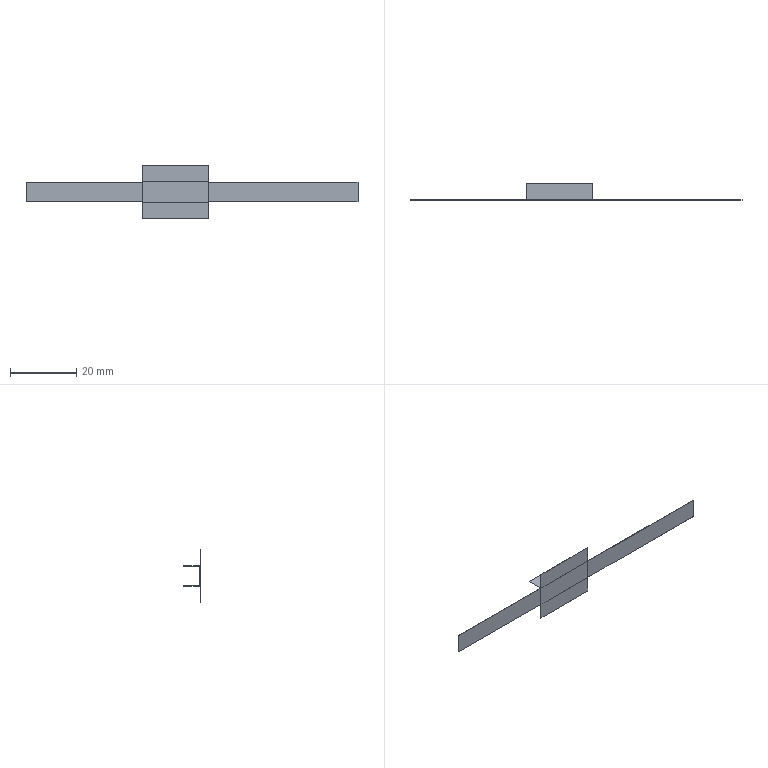Part | SolidWorks | features ICE 2, ExtruThin 1 | 1 solid | 22 faces | box 100 x 5.02 x 16 mm | volume 70.4 mm3 | plane 22
STEP:
#1=CARTESIAN_POINT('',(35.,0.05,3.));
#2=VERTEX_POINT('',#1);
#3=CARTESIAN_POINT('',(35.,-0.05,3.));
#4=VERTEX_POINT('',#3);
#5=CARTESIAN_POINT('',(35.,4.95,3.));
#6=DIRECTION('',(0.,-1.,0.));
#7=VECTOR('',#6,1000.);
#8=LINE('',#5,#7);
#9=EDGE_CURVE('',#2,#4,#8,.T.);
#10=ORIENTED_EDGE('',*,*,#9,.F.);
#11=CARTESIAN_POINT('',(0.,0.05,3.));
#12=VERTEX_POINT('',#11);
#13=CARTESIAN_POINT('',(0.,0.05,3.));
#14=DIRECTION('',(1.,0.,0.));
#15=VECTOR('',#14,1000.);
#16=LINE('',#13,#15);
#17=EDGE_CURVE('',#12,#2,#16,.T.);
#18=ORIENTED_EDGE('',*,*,#17,.F.);
#19=CARTESIAN_POINT('',(0.,-0.05,3.));
#20=VERTEX_POINT('',#19);
#21=CARTESIAN_POINT('',(0.,-0.05,3.));
#22=DIRECTION('',(0.,1.,0.));
#23=VECTOR('',#22,1000.);
#24=LINE('',#21,#23);
#25=EDGE_CURVE('',#20,#12,#24,.T.);
#26=ORIENTED_EDGE('',*,*,#25,.F.);
#27=CARTESIAN_POINT('',(0.,-0.05,3.));
#28=DIRECTION('',(1.,0.,0.));
#29=VECTOR('',#28,1000.);
#30=LINE('',#27,#29);
#31=EDGE_CURVE('',#20,#4,#30,.T.);
#32=ORIENTED_EDGE('',*,*,#31,.T.);
#33=EDGE_LOOP('',(#10,#18,#26,#32));
#34=FACE_OUTER_BOUND('',#33,.T.);
#35=CARTESIAN_POINT('',(100.,-0.05,3.));
#36=DIRECTION('',(0.,0.,-1.));
#37=DIRECTION('',(-1.,0.,0.));
#38=AXIS2_PLACEMENT_3D('',#35,#36,#37);
#39=PLANE('',#38);
#40=ADVANCED_FACE('',(#34),#39,.F.);
#41=CARTESIAN_POINT('',(55.,0.05,3.));
#42=VERTEX_POINT('',#41);
#43=CARTESIAN_POINT('',(55.,-0.05,3.));
#44=VERTEX_POINT('',#43);
#45=CARTESIAN_POINT('',(55.,4.95,3.));
#46=DIRECTION('',(0.,-1.,0.));
#47=VECTOR('',#46,1000.);
#48=LINE('',#45,#47);
#49=EDGE_CURVE('',#42,#44,#48,.T.);
#50=ORIENTED_EDGE('',*,*,#49,.T.);
#51=CARTESIAN_POINT('',(100.,-0.05,3.));
#52=VERTEX_POINT('',#51);
#53=CARTESIAN_POINT('',(0.,-0.05,3.));
#54=DIRECTION('',(1.,0.,0.));
#55=VECTOR('',#54,1000.);
#56=LINE('',#53,#55);
#57=EDGE_CURVE('',#44,#52,#56,.T.);
#58=ORIENTED_EDGE('',*,*,#57,.T.);
#59=CARTESIAN_POINT('',(100.,0.05,3.));
#60=VERTEX_POINT('',#59);
#61=CARTESIAN_POINT('',(100.,0.05,3.));
#62=DIRECTION('',(0.,-1.,0.));
#63=VECTOR('',#62,1000.);
#64=LINE('',#61,#63);
#65=EDGE_CURVE('',#60,#52,#64,.T.);
#66=ORIENTED_EDGE('',*,*,#65,.F.);
#67=CARTESIAN_POINT('',(0.,0.05,3.));
#68=DIRECTION('',(1.,0.,0.));
#69=VECTOR('',#68,1000.);
#70=LINE('',#67,#69);
#71=EDGE_CURVE('',#42,#60,#70,.T.);
#72=ORIENTED_EDGE('',*,*,#71,.F.);
#73=EDGE_LOOP('',(#50,#58,#66,#72));
#74=FACE_OUTER_BOUND('',#73,.T.);
#75=CARTESIAN_POINT('',(100.,-0.05,3.));
#76=DIRECTION('',(0.,0.,-1.));
#77=DIRECTION('',(-1.,0.,0.));
#78=AXIS2_PLACEMENT_3D('',#75,#76,#77);
#79=PLANE('',#78);
#80=ADVANCED_FACE('',(#74),#79,.F.);
#81=CARTESIAN_POINT('',(55.,-0.05,3.02));
#82=VERTEX_POINT('',#81);
#83=CARTESIAN_POINT('',(55.,-0.05,8.));
#84=VERTEX_POINT('',#83);
#85=CARTESIAN_POINT('',(55.,-0.05,-8.));
#86=DIRECTION('',(0.,0.,1.));
#87=VECTOR('',#86,1000.);
#88=LINE('',#85,#87);
#89=EDGE_CURVE('',#82,#84,#88,.T.);
#90=ORIENTED_EDGE('',*,*,#89,.F.);
#91=CARTESIAN_POINT('',(35.,-0.05,3.02));
#92=VERTEX_POINT('',#91);
#93=CARTESIAN_POINT('',(35.,-0.05,3.02));
#94=DIRECTION('',(1.,0.,0.));
#95=VECTOR('',#94,1000.);
#96=LINE('',#93,#95);
#97=EDGE_CURVE('',#92,#82,#96,.T.);
#98=ORIENTED_EDGE('',*,*,#97,.F.);
#99=CARTESIAN_POINT('',(35.,-0.05,8.));
#100=VERTEX_POINT('',#99);
#101=CARTESIAN_POINT('',(35.,-0.05,-8.));
#102=DIRECTION('',(0.,0.,-1.));
#103=VECTOR('',#102,1000.);
#104=LINE('',#101,#103);
#105=EDGE_CURVE('',#100,#92,#104,.T.);
#106=ORIENTED_EDGE('',*,*,#105,.F.);
#107=CARTESIAN_POINT('',(35.,-0.05,8.));
#108=DIRECTION('',(-1.,0.,0.));
#109=VECTOR('',#108,1000.);
#110=LINE('',#107,#109);
#111=EDGE_CURVE('',#84,#100,#110,.T.);
#112=ORIENTED_EDGE('',*,*,#111,.F.);
#113=EDGE_LOOP('',(#90,#98,#106,#112));
#114=FACE_OUTER_BOUND('',#113,.T.);
#115=CARTESIAN_POINT('',(55.,-0.05,8.));
#116=DIRECTION('',(0.,1.,0.));
#117=DIRECTION('',(0.,0.,1.));
#118=AXIS2_PLACEMENT_3D('',#115,#116,#117);
#119=PLANE('',#118);
#120=ADVANCED_FACE('',(#114),#119,.T.);
#121=CARTESIAN_POINT('',(0.,0.05,-3.));
#122=VERTEX_POINT('',#121);
#123=CARTESIAN_POINT('',(35.,0.05,-3.));
#124=VERTEX_POINT('',#123);
#125=CARTESIAN_POINT('',(0.,0.05,-3.));
#126=DIRECTION('',(1.,0.,0.));
#127=VECTOR('',#126,1000.);
#128=LINE('',#125,#127);
#129=EDGE_CURVE('',#122,#124,#128,.T.);
#130=ORIENTED_EDGE('',*,*,#129,.T.);
#131=CARTESIAN_POINT('',(35.,-0.05,-3.));
#132=VERTEX_POINT('',#131);
#133=CARTESIAN_POINT('',(35.,4.95,-3.));
#134=DIRECTION('',(0.,-1.,0.));
#135=VECTOR('',#134,1000.);
#136=LINE('',#133,#135);
#137=EDGE_CURVE('',#124,#132,#136,.T.);
#138=ORIENTED_EDGE('',*,*,#137,.T.);
#139=CARTESIAN_POINT('',(0.,-0.05,-3.));
#140=VERTEX_POINT('',#139);
#141=CARTESIAN_POINT('',(0.,-0.05,-3.));
#142=DIRECTION('',(1.,0.,0.));
#143=VECTOR('',#142,1000.);
#144=LINE('',#141,#143);
#145=EDGE_CURVE('',#140,#132,#144,.T.);
#146=ORIENTED_EDGE('',*,*,#145,.F.);
#147=CARTESIAN_POINT('',(0.,-0.05,-3.));
#148=DIRECTION('',(0.,1.,0.));
#149=VECTOR('',#148,1000.);
#150=LINE('',#147,#149);
#151=EDGE_CURVE('',#140,#122,#150,.T.);
#152=ORIENTED_EDGE('',*,*,#151,.T.);
#153=EDGE_LOOP('',(#130,#138,#146,#152));
#154=FACE_OUTER_BOUND('',#153,.T.);
#155=CARTESIAN_POINT('',(100.,-0.05,-3.));
#156=DIRECTION('',(0.,0.,-1.));
#157=DIRECTION('',(-1.,0.,0.));
#158=AXIS2_PLACEMENT_3D('',#155,#156,#157);
#159=PLANE('',#158);
#160=ADVANCED_FACE('',(#154),#159,.T.);
#161=CARTESIAN_POINT('',(55.,-0.05,-3.));
#162=VERTEX_POINT('',#161);
#163=CARTESIAN_POINT('',(100.,-0.05,-3.));
#164=VERTEX_POINT('',#163);
#165=CARTESIAN_POINT('',(0.,-0.05,-3.));
#166=DIRECTION('',(1.,0.,0.));
#167=VECTOR('',#166,1000.);
#168=LINE('',#165,#167);
#169=EDGE_CURVE('',#162,#164,#168,.T.);
#170=ORIENTED_EDGE('',*,*,#169,.F.);
#171=CARTESIAN_POINT('',(55.,0.05,-3.));
#172=VERTEX_POINT('',#171);
#173=CARTESIAN_POINT('',(55.,4.95,-3.));
#174=DIRECTION('',(0.,-1.,0.));
#175=VECTOR('',#174,1000.);
#176=LINE('',#173,#175);
#177=EDGE_CURVE('',#172,#162,#176,.T.);
#178=ORIENTED_EDGE('',*,*,#177,.F.);
#179=CARTESIAN_POINT('',(100.,0.05,-3.));
#180=VERTEX_POINT('',#179);
#181=CARTESIAN_POINT('',(0.,0.05,-3.));
#182=DIRECTION('',(1.,0.,0.));
#183=VECTOR('',#182,1000.);
#184=LINE('',#181,#183);
#185=EDGE_CURVE('',#172,#180,#184,.T.);
#186=ORIENTED_EDGE('',*,*,#185,.T.);
#187=CARTESIAN_POINT('',(100.,0.05,-3.));
#188=DIRECTION('',(0.,-1.,0.));
#189=VECTOR('',#188,1000.);
#190=LINE('',#187,#189);
#191=EDGE_CURVE('',#180,#164,#190,.T.);
#192=ORIENTED_EDGE('',*,*,#191,.T.);
#193=EDGE_LOOP('',(#170,#178,#186,#192));
#194=FACE_OUTER_BOUND('',#193,.T.);
#195=CARTESIAN_POINT('',(100.,-0.05,-3.));
#196=DIRECTION('',(0.,0.,-1.));
#197=DIRECTION('',(-1.,0.,0.));
#198=AXIS2_PLACEMENT_3D('',#195,#196,#197);
#199=PLANE('',#198);
#200=ADVANCED_FACE('',(#194),#199,.T.);
#201=CARTESIAN_POINT('',(35.,-0.05,-3.02));
#202=VERTEX_POINT('',#201);
#203=CARTESIAN_POINT('',(35.,-0.05,-8.));
#204=VERTEX_POINT('',#203);
#205=CARTESIAN_POINT('',(35.,-0.05,-8.));
#206=DIRECTION('',(0.,0.,-1.));
#207=VECTOR('',#206,1000.);
#208=LINE('',#205,#207);
#209=EDGE_CURVE('',#202,#204,#208,.T.);
#210=ORIENTED_EDGE('',*,*,#209,.F.);
#211=CARTESIAN_POINT('',(55.,-0.05,-3.02));
#212=VERTEX_POINT('',#211);
#213=CARTESIAN_POINT('',(35.,-0.05,-3.02));
#214=DIRECTION('',(-1.,0.,0.));
#215=VECTOR('',#214,1000.);
#216=LINE('',#213,#215);
#217=EDGE_CURVE('',#212,#202,#216,.T.);
#218=ORIENTED_EDGE('',*,*,#217,.F.);
#219=CARTESIAN_POINT('',(55.,-0.05,-8.));
#220=VERTEX_POINT('',#219);
#221=CARTESIAN_POINT('',(55.,-0.05,-8.));
#222=DIRECTION('',(0.,0.,1.));
#223=VECTOR('',#222,1000.);
#224=LINE('',#221,#223);
#225=EDGE_CURVE('',#220,#212,#224,.T.);
#226=ORIENTED_EDGE('',*,*,#225,.F.);
#227=CARTESIAN_POINT('',(35.,-0.05,-8.));
#228=DIRECTION('',(1.,0.,0.));
#229=VECTOR('',#228,1000.);
#230=LINE('',#227,#229);
#231=EDGE_CURVE('',#204,#220,#230,.T.);
#232=ORIENTED_EDGE('',*,*,#231,.F.);
#233=EDGE_LOOP('',(#210,#218,#226,#232));
#234=FACE_OUTER_BOUND('',#233,.T.);
#235=CARTESIAN_POINT('',(55.,-0.05,8.));
#236=DIRECTION('',(0.,1.,0.));
#237=DIRECTION('',(0.,0.,1.));
#238=AXIS2_PLACEMENT_3D('',#235,#236,#237);
#239=PLANE('',#238);
#240=ADVANCED_FACE('',(#234),#239,.T.);
#241=CARTESIAN_POINT('',(55.,-0.05,-8.));
#242=DIRECTION('',(0.,0.,1.));
#243=VECTOR('',#242,1000.);
#244=LINE('',#241,#243);
#245=EDGE_CURVE('',#162,#44,#244,.T.);
#246=ORIENTED_EDGE('',*,*,#245,.F.);
#247=ORIENTED_EDGE('',*,*,#169,.T.);
#248=CARTESIAN_POINT('',(100.,-0.05,3.));
#249=DIRECTION('',(0.,0.,-1.));
#250=VECTOR('',#249,1000.);
#251=LINE('',#248,#250);
#252=EDGE_CURVE('',#52,#164,#251,.T.);
#253=ORIENTED_EDGE('',*,*,#252,.F.);
#254=ORIENTED_EDGE('',*,*,#57,.F.);
#255=EDGE_LOOP('',(#246,#247,#253,#254));
#256=FACE_OUTER_BOUND('',#255,.T.);
#257=CARTESIAN_POINT('',(0.,-0.05,3.));
#258=DIRECTION('',(0.,1.,0.));
#259=DIRECTION('',(0.,0.,1.));
#260=AXIS2_PLACEMENT_3D('',#257,#258,#259);
#261=PLANE('',#260);
#262=ADVANCED_FACE('',(#256),#261,.F.);
#263=CARTESIAN_POINT('',(35.,-0.05,-8.));
#264=DIRECTION('',(0.,0.,-1.));
#265=VECTOR('',#264,1000.);
#266=LINE('',#263,#265);
#267=EDGE_CURVE('',#4,#132,#266,.T.);
#268=ORIENTED_EDGE('',*,*,#267,.F.);
#269=ORIENTED_EDGE('',*,*,#31,.F.);
#270=CARTESIAN_POINT('',(0.,-0.05,3.));
#271=DIRECTION('',(0.,0.,-1.));
#272=VECTOR('',#271,1000.);
#273=LINE('',#270,#272);
#274=EDGE_CURVE('',#20,#140,#273,.T.);
#275=ORIENTED_EDGE('',*,*,#274,.T.);
#276=ORIENTED_EDGE('',*,*,#145,.T.);
#277=EDGE_LOOP('',(#268,#269,#275,#276));
#278=FACE_OUTER_BOUND('',#277,.T.);
#279=CARTESIAN_POINT('',(0.,-0.05,3.));
#280=DIRECTION('',(0.,1.,0.));
#281=DIRECTION('',(0.,0.,1.));
#282=AXIS2_PLACEMENT_3D('',#279,#280,#281);
#283=PLANE('',#282);
#284=ADVANCED_FACE('',(#278),#283,.F.);
#285=ORIENTED_EDGE('',*,*,#191,.F.);
#286=CARTESIAN_POINT('',(100.,0.05,3.));
#287=DIRECTION('',(0.,0.,-1.));
#288=VECTOR('',#287,1000.);
#289=LINE('',#286,#288);
#290=EDGE_CURVE('',#60,#180,#289,.T.);
#291=ORIENTED_EDGE('',*,*,#290,.F.);
#292=ORIENTED_EDGE('',*,*,#65,.T.);
#293=ORIENTED_EDGE('',*,*,#252,.T.);
#294=EDGE_LOOP('',(#285,#291,#292,#293));
#295=FACE_OUTER_BOUND('',#294,.T.);
#296=CARTESIAN_POINT('',(100.,0.05,3.));
#297=DIRECTION('',(1.,0.,0.));
#298=DIRECTION('',(0.,0.,-1.));
#299=AXIS2_PLACEMENT_3D('',#296,#297,#298);
#300=PLANE('',#299);
#301=ADVANCED_FACE('',(#295),#300,.T.);
#302=ORIENTED_EDGE('',*,*,#129,.F.);
#303=CARTESIAN_POINT('',(0.,0.05,3.));
#304=DIRECTION('',(0.,0.,-1.));
#305=VECTOR('',#304,1000.);
#306=LINE('',#303,#305);
#307=EDGE_CURVE('',#12,#122,#306,.T.);
#308=ORIENTED_EDGE('',*,*,#307,.F.);
#309=ORIENTED_EDGE('',*,*,#17,.T.);
#310=CARTESIAN_POINT('',(0.,0.05,3.));
#311=DIRECTION('',(1.,0.,0.));
#312=VECTOR('',#311,1000.);
#313=LINE('',#310,#312);
#314=EDGE_CURVE('',#2,#42,#313,.T.);
#315=ORIENTED_EDGE('',*,*,#314,.T.);
#316=ORIENTED_EDGE('',*,*,#71,.T.);
#317=ORIENTED_EDGE('',*,*,#290,.T.);
#318=ORIENTED_EDGE('',*,*,#185,.F.);
#319=CARTESIAN_POINT('',(0.,0.05,-3.));
#320=DIRECTION('',(-1.,0.,0.));
#321=VECTOR('',#320,1000.);
#322=LINE('',#319,#321);
#323=EDGE_CURVE('',#172,#124,#322,.T.);
#324=ORIENTED_EDGE('',*,*,#323,.T.);
#325=EDGE_LOOP('',(#302,#308,#309,#315,#316,#317,#318,#324));
#326=FACE_OUTER_BOUND('',#325,.T.);
#327=CARTESIAN_POINT('',(0.,0.05,3.));
#328=DIRECTION('',(0.,1.,0.));
#329=DIRECTION('',(0.,0.,1.));
#330=AXIS2_PLACEMENT_3D('',#327,#328,#329);
#331=PLANE('',#330);
#332=ADVANCED_FACE('',(#326),#331,.T.);
#333=ORIENTED_EDGE('',*,*,#151,.F.);
#334=ORIENTED_EDGE('',*,*,#274,.F.);
#335=ORIENTED_EDGE('',*,*,#25,.T.);
#336=ORIENTED_EDGE('',*,*,#307,.T.);
#337=EDGE_LOOP('',(#333,#334,#335,#336));
#338=FACE_OUTER_BOUND('',#337,.T.);
#339=CARTESIAN_POINT('',(0.,-0.05,3.));
#340=DIRECTION('',(-1.,0.,0.));
#341=DIRECTION('',(0.,0.,1.));
#342=AXIS2_PLACEMENT_3D('',#339,#340,#341);
#343=PLANE('',#342);
#344=ADVANCED_FACE('',(#338),#343,.T.);
#345=ORIENTED_EDGE('',*,*,#225,.T.);
#346=CARTESIAN_POINT('',(55.,4.95,-3.02));
#347=VERTEX_POINT('',#346);
#348=CARTESIAN_POINT('',(55.,4.95,-3.02));
#349=DIRECTION('',(0.,-1.,0.));
#350=VECTOR('',#349,1000.);
#351=LINE('',#348,#350);
#352=EDGE_CURVE('',#347,#212,#351,.T.);
#353=ORIENTED_EDGE('',*,*,#352,.F.);
#354=CARTESIAN_POINT('',(55.,4.95,-3.));
#355=VERTEX_POINT('',#354);
#356=CARTESIAN_POINT('',(55.,4.95,-3.));
#357=DIRECTION('',(0.,0.,-1.));
#358=VECTOR('',#357,1000.);
#359=LINE('',#356,#358);
#360=EDGE_CURVE('',#355,#347,#359,.T.);
#361=ORIENTED_EDGE('',*,*,#360,.F.);
#362=CARTESIAN_POINT('',(55.,4.95,-3.));
#363=DIRECTION('',(0.,-1.,0.));
#364=VECTOR('',#363,1000.);
#365=LINE('',#362,#364);
#366=EDGE_CURVE('',#355,#172,#365,.T.);
#367=ORIENTED_EDGE('',*,*,#366,.T.);
#368=ORIENTED_EDGE('',*,*,#177,.T.);
#369=ORIENTED_EDGE('',*,*,#245,.T.);
#370=ORIENTED_EDGE('',*,*,#49,.F.);
#371=CARTESIAN_POINT('',(55.,4.95,3.));
#372=VERTEX_POINT('',#371);
#373=CARTESIAN_POINT('',(55.,4.95,3.));
#374=DIRECTION('',(0.,-1.,0.));
#375=VECTOR('',#374,1000.);
#376=LINE('',#373,#375);
#377=EDGE_CURVE('',#372,#42,#376,.T.);
#378=ORIENTED_EDGE('',*,*,#377,.F.);
#379=CARTESIAN_POINT('',(55.,4.95,3.02));
#380=VERTEX_POINT('',#379);
#381=CARTESIAN_POINT('',(55.,4.95,3.));
#382=DIRECTION('',(0.,0.,-1.));
#383=VECTOR('',#382,1000.);
#384=LINE('',#381,#383);
#385=EDGE_CURVE('',#380,#372,#384,.T.);
#386=ORIENTED_EDGE('',*,*,#385,.F.);
#387=CARTESIAN_POINT('',(55.,4.95,3.02));
#388=DIRECTION('',(0.,-1.,0.));
#389=VECTOR('',#388,1000.);
#390=LINE('',#387,#389);
#391=EDGE_CURVE('',#380,#82,#390,.T.);
#392=ORIENTED_EDGE('',*,*,#391,.T.);
#393=ORIENTED_EDGE('',*,*,#89,.T.);
#394=CARTESIAN_POINT('',(55.,-0.07,8.));
#395=VERTEX_POINT('',#394);
#396=CARTESIAN_POINT('',(55.,-0.07,8.));
#397=DIRECTION('',(0.,1.,0.));
#398=VECTOR('',#397,1000.);
#399=LINE('',#396,#398);
#400=EDGE_CURVE('',#395,#84,#399,.T.);
#401=ORIENTED_EDGE('',*,*,#400,.F.);
#402=CARTESIAN_POINT('',(55.,-0.07,-8.));
#403=VERTEX_POINT('',#402);
#404=CARTESIAN_POINT('',(55.,-0.07,-8.));
#405=DIRECTION('',(0.,0.,1.));
#406=VECTOR('',#405,1000.);
#407=LINE('',#404,#406);
#408=EDGE_CURVE('',#403,#395,#407,.T.);
#409=ORIENTED_EDGE('',*,*,#408,.F.);
#410=CARTESIAN_POINT('',(55.,-0.07,-8.));
#411=DIRECTION('',(0.,1.,0.));
#412=VECTOR('',#411,1000.);
#413=LINE('',#410,#412);
#414=EDGE_CURVE('',#403,#220,#413,.T.);
#415=ORIENTED_EDGE('',*,*,#414,.T.);
#416=EDGE_LOOP('',(#345,#353,#361,#367,#368,#369,#370,#378,#386,#392,#393,#401,#409,#415));
#417=FACE_OUTER_BOUND('',#416,.T.);
#418=CARTESIAN_POINT('',(55.,-0.07,-8.));
#419=DIRECTION('',(-1.,0.,0.));
#420=DIRECTION('',(0.,0.,1.));
#421=AXIS2_PLACEMENT_3D('',#418,#419,#420);
#422=PLANE('',#421);
#423=ADVANCED_FACE('',(#417),#422,.F.);
#424=ORIENTED_EDGE('',*,*,#111,.T.);
#425=CARTESIAN_POINT('',(35.,-0.07,8.));
#426=VERTEX_POINT('',#425);
#427=CARTESIAN_POINT('',(35.,-0.07,8.));
#428=DIRECTION('',(0.,1.,0.));
#429=VECTOR('',#428,1000.);
#430=LINE('',#427,#429);
#431=EDGE_CURVE('',#426,#100,#430,.T.);
#432=ORIENTED_EDGE('',*,*,#431,.F.);
#433=CARTESIAN_POINT('',(35.,-0.07,8.));
#434=DIRECTION('',(-1.,0.,0.));
#435=VECTOR('',#434,1000.);
#436=LINE('',#433,#435);
#437=EDGE_CURVE('',#395,#426,#436,.T.);
#438=ORIENTED_EDGE('',*,*,#437,.F.);
#439=ORIENTED_EDGE('',*,*,#400,.T.);
#440=EDGE_LOOP('',(#424,#432,#438,#439));
#441=FACE_OUTER_BOUND('',#440,.T.);
#442=CARTESIAN_POINT('',(35.,-0.07,8.));
#443=DIRECTION('',(0.,0.,-1.));
#444=DIRECTION('',(-1.,0.,0.));
#445=AXIS2_PLACEMENT_3D('',#442,#443,#444);
#446=PLANE('',#445);
#447=ADVANCED_FACE('',(#441),#446,.F.);
#448=ORIENTED_EDGE('',*,*,#105,.T.);
#449=CARTESIAN_POINT('',(35.,4.95,3.02));
#450=VERTEX_POINT('',#449);
#451=CARTESIAN_POINT('',(35.,4.95,3.02));
#452=DIRECTION('',(0.,-1.,0.));
#453=VECTOR('',#452,1000.);
#454=LINE('',#451,#453);
#455=EDGE_CURVE('',#450,#92,#454,.T.);
#456=ORIENTED_EDGE('',*,*,#455,.F.);
#457=CARTESIAN_POINT('',(35.,4.95,3.));
#458=VERTEX_POINT('',#457);
#459=CARTESIAN_POINT('',(35.,4.95,3.));
#460=DIRECTION('',(0.,0.,1.));
#461=VECTOR('',#460,1000.);
#462=LINE('',#459,#461);
#463=EDGE_CURVE('',#458,#450,#462,.T.);
#464=ORIENTED_EDGE('',*,*,#463,.F.);
#465=CARTESIAN_POINT('',(35.,4.95,3.));
#466=DIRECTION('',(0.,-1.,0.));
#467=VECTOR('',#466,1000.);
#468=LINE('',#465,#467);
#469=EDGE_CURVE('',#458,#2,#468,.T.);
#470=ORIENTED_EDGE('',*,*,#469,.T.);
#471=ORIENTED_EDGE('',*,*,#9,.T.);
#472=ORIENTED_EDGE('',*,*,#267,.T.);
#473=ORIENTED_EDGE('',*,*,#137,.F.);
#474=CARTESIAN_POINT('',(35.,4.95,-3.));
#475=VERTEX_POINT('',#474);
#476=CARTESIAN_POINT('',(35.,4.95,-3.));
#477=DIRECTION('',(0.,-1.,0.));
#478=VECTOR('',#477,1000.);
#479=LINE('',#476,#478);
#480=EDGE_CURVE('',#475,#124,#479,.T.);
#481=ORIENTED_EDGE('',*,*,#480,.F.);
#482=CARTESIAN_POINT('',(35.,4.95,-3.02));
#483=VERTEX_POINT('',#482);
#484=CARTESIAN_POINT('',(35.,4.95,-3.));
#485=DIRECTION('',(0.,0.,1.));
#486=VECTOR('',#485,1000.);
#487=LINE('',#484,#486);
#488=EDGE_CURVE('',#483,#475,#487,.T.);
#489=ORIENTED_EDGE('',*,*,#488,.F.);
#490=CARTESIAN_POINT('',(35.,4.95,-3.02));
#491=DIRECTION('',(0.,-1.,0.));
#492=VECTOR('',#491,1000.);
#493=LINE('',#490,#492);
#494=EDGE_CURVE('',#483,#202,#493,.T.);
#495=ORIENTED_EDGE('',*,*,#494,.T.);
#496=ORIENTED_EDGE('',*,*,#209,.T.);
#497=CARTESIAN_POINT('',(35.,-0.07,-8.));
#498=VERTEX_POINT('',#497);
#499=CARTESIAN_POINT('',(35.,-0.07,-8.));
#500=DIRECTION('',(0.,1.,0.));
#501=VECTOR('',#500,1000.);
#502=LINE('',#499,#501);
#503=EDGE_CURVE('',#498,#204,#502,.T.);
#504=ORIENTED_EDGE('',*,*,#503,.F.);
#505=CARTESIAN_POINT('',(35.,-0.07,-8.));
#506=DIRECTION('',(0.,0.,-1.));
#507=VECTOR('',#506,1000.);
#508=LINE('',#505,#507);
#509=EDGE_CURVE('',#426,#498,#508,.T.);
#510=ORIENTED_EDGE('',*,*,#509,.F.);
#511=ORIENTED_EDGE('',*,*,#431,.T.);
#512=EDGE_LOOP('',(#448,#456,#464,#470,#471,#472,#473,#481,#489,#495,#496,#504,#510,#511));
#513=FACE_OUTER_BOUND('',#512,.T.);
#514=CARTESIAN_POINT('',(35.,-0.07,-8.));
#515=DIRECTION('',(1.,0.,0.));
#516=DIRECTION('',(0.,0.,-1.));
#517=AXIS2_PLACEMENT_3D('',#514,#515,#516);
#518=PLANE('',#517);
#519=ADVANCED_FACE('',(#513),#518,.F.);
#520=ORIENTED_EDGE('',*,*,#231,.T.);
#521=ORIENTED_EDGE('',*,*,#414,.F.);
#522=CARTESIAN_POINT('',(35.,-0.07,-8.));
#523=DIRECTION('',(1.,0.,0.));
#524=VECTOR('',#523,1000.);
#525=LINE('',#522,#524);
#526=EDGE_CURVE('',#498,#403,#525,.T.);
#527=ORIENTED_EDGE('',*,*,#526,.F.);
#528=ORIENTED_EDGE('',*,*,#503,.T.);
#529=EDGE_LOOP('',(#520,#521,#527,#528));
#530=FACE_OUTER_BOUND('',#529,.T.);
#531=CARTESIAN_POINT('',(35.,-0.07,-8.));
#532=DIRECTION('',(0.,0.,1.));
#533=DIRECTION('',(1.,0.,0.));
#534=AXIS2_PLACEMENT_3D('',#531,#532,#533);
#535=PLANE('',#534);
#536=ADVANCED_FACE('',(#530),#535,.F.);
#537=ORIENTED_EDGE('',*,*,#408,.T.);
#538=ORIENTED_EDGE('',*,*,#437,.T.);
#539=ORIENTED_EDGE('',*,*,#509,.T.);
#540=ORIENTED_EDGE('',*,*,#526,.T.);
#541=EDGE_LOOP('',(#537,#538,#539,#540));
#542=FACE_OUTER_BOUND('',#541,.T.);
#543=CARTESIAN_POINT('',(55.,-0.07,8.));
#544=DIRECTION('',(0.,1.,0.));
#545=DIRECTION('',(0.,0.,1.));
#546=AXIS2_PLACEMENT_3D('',#543,#544,#545);
#547=PLANE('',#546);
#548=ADVANCED_FACE('',(#542),#547,.F.);
#549=ORIENTED_EDGE('',*,*,#323,.F.);
#550=ORIENTED_EDGE('',*,*,#366,.F.);
#551=CARTESIAN_POINT('',(35.,4.95,-3.));
#552=DIRECTION('',(1.,0.,0.));
#553=VECTOR('',#552,1000.);
#554=LINE('',#551,#553);
#555=EDGE_CURVE('',#475,#355,#554,.T.);
#556=ORIENTED_EDGE('',*,*,#555,.F.);
#557=ORIENTED_EDGE('',*,*,#480,.T.);
#558=EDGE_LOOP('',(#549,#550,#556,#557));
#559=FACE_OUTER_BOUND('',#558,.T.);
#560=CARTESIAN_POINT('',(35.,4.95,-3.));
#561=DIRECTION('',(0.,0.,-1.));
#562=DIRECTION('',(-1.,0.,0.));
#563=AXIS2_PLACEMENT_3D('',#560,#561,#562);
#564=PLANE('',#563);
#565=ADVANCED_FACE('',(#559),#564,.F.);
#566=ORIENTED_EDGE('',*,*,#217,.T.);
#567=ORIENTED_EDGE('',*,*,#494,.F.);
#568=CARTESIAN_POINT('',(35.,4.95,-3.02));
#569=DIRECTION('',(-1.,0.,0.));
#570=VECTOR('',#569,1000.);
#571=LINE('',#568,#570);
#572=EDGE_CURVE('',#347,#483,#571,.T.);
#573=ORIENTED_EDGE('',*,*,#572,.F.);
#574=ORIENTED_EDGE('',*,*,#352,.T.);
#575=EDGE_LOOP('',(#566,#567,#573,#574));
#576=FACE_OUTER_BOUND('',#575,.T.);
#577=CARTESIAN_POINT('',(35.,4.95,-3.02));
#578=DIRECTION('',(0.,0.,1.));
#579=DIRECTION('',(1.,0.,0.));
#580=AXIS2_PLACEMENT_3D('',#577,#578,#579);
#581=PLANE('',#580);
#582=ADVANCED_FACE('',(#576),#581,.F.);
#583=ORIENTED_EDGE('',*,*,#488,.T.);
#584=ORIENTED_EDGE('',*,*,#555,.T.);
#585=ORIENTED_EDGE('',*,*,#360,.T.);
#586=ORIENTED_EDGE('',*,*,#572,.T.);
#587=EDGE_LOOP('',(#583,#584,#585,#586));
#588=FACE_OUTER_BOUND('',#587,.T.);
#589=CARTESIAN_POINT('',(35.,4.95,-3.02));
#590=DIRECTION('',(0.,-1.,0.));
#591=DIRECTION('',(0.,0.,-1.));
#592=AXIS2_PLACEMENT_3D('',#589,#590,#591);
#593=PLANE('',#592);
#594=ADVANCED_FACE('',(#588),#593,.F.);
#595=ORIENTED_EDGE('',*,*,#314,.F.);
#596=ORIENTED_EDGE('',*,*,#469,.F.);
#597=CARTESIAN_POINT('',(35.,4.95,3.));
#598=DIRECTION('',(-1.,0.,0.));
#599=VECTOR('',#598,1000.);
#600=LINE('',#597,#599);
#601=EDGE_CURVE('',#372,#458,#600,.T.);
#602=ORIENTED_EDGE('',*,*,#601,.F.);
#603=ORIENTED_EDGE('',*,*,#377,.T.);
#604=EDGE_LOOP('',(#595,#596,#602,#603));
#605=FACE_OUTER_BOUND('',#604,.T.);
#606=CARTESIAN_POINT('',(35.,4.95,3.));
#607=DIRECTION('',(0.,0.,1.));
#608=DIRECTION('',(1.,0.,0.));
#609=AXIS2_PLACEMENT_3D('',#606,#607,#608);
#610=PLANE('',#609);
#611=ADVANCED_FACE('',(#605),#610,.F.);
#612=ORIENTED_EDGE('',*,*,#97,.T.);
#613=ORIENTED_EDGE('',*,*,#391,.F.);
#614=CARTESIAN_POINT('',(35.,4.95,3.02));
#615=DIRECTION('',(1.,0.,0.));
#616=VECTOR('',#615,1000.);
#617=LINE('',#614,#616);
#618=EDGE_CURVE('',#450,#380,#617,.T.);
#619=ORIENTED_EDGE('',*,*,#618,.F.);
#620=ORIENTED_EDGE('',*,*,#455,.T.);
#621=EDGE_LOOP('',(#612,#613,#619,#620));
#622=FACE_OUTER_BOUND('',#621,.T.);
#623=CARTESIAN_POINT('',(35.,4.95,3.02));
#624=DIRECTION('',(0.,0.,-1.));
#625=DIRECTION('',(-1.,0.,0.));
#626=AXIS2_PLACEMENT_3D('',#623,#624,#625);
#627=PLANE('',#626);
#628=ADVANCED_FACE('',(#622),#627,.F.);
#629=ORIENTED_EDGE('',*,*,#601,.T.);
#630=ORIENTED_EDGE('',*,*,#463,.T.);
#631=ORIENTED_EDGE('',*,*,#618,.T.);
#632=ORIENTED_EDGE('',*,*,#385,.T.);
#633=EDGE_LOOP('',(#629,#630,#631,#632));
#634=FACE_OUTER_BOUND('',#633,.T.);
#635=CARTESIAN_POINT('',(55.,4.95,3.));
#636=DIRECTION('',(0.,-1.,0.));
#637=DIRECTION('',(0.,0.,-1.));
#638=AXIS2_PLACEMENT_3D('',#635,#636,#637);
#639=PLANE('',#638);
#640=ADVANCED_FACE('',(#634),#639,.F.);
#641=CLOSED_SHELL('',(#40,#80,#120,#160,#200,#240,#262,#284,#301,#332,#344,#423,#447,#519,#536,#548,#565,#582,#594,#611,#628,#640));
#642=MANIFOLD_SOLID_BREP('',#641);
#643=CARTESIAN_POINT('',(0.,0.,0.));
#644=DIRECTION('',(0.,0.,1.));
#645=DIRECTION('',(1.,0.,0.));
#646=AXIS2_PLACEMENT_3D('',#643,#644,#645);
#647=(LENGTH_UNIT()NAMED_UNIT(*)SI_UNIT(.MILLI.,.METRE.));
#648=UNCERTAINTY_MEASURE_WITH_UNIT(LENGTH_MEASURE(0.00001),#647,'','');
#649=(NAMED_UNIT(*)PLANE_ANGLE_UNIT()SI_UNIT($,.RADIAN.));
#650=(NAMED_UNIT(*)SI_UNIT($,.STERADIAN.)SOLID_ANGLE_UNIT());
#651=(GEOMETRIC_REPRESENTATION_CONTEXT(3)GLOBAL_UNCERTAINTY_ASSIGNED_CONTEXT((#648))GLOBAL_UNIT_ASSIGNED_CONTEXT((#647,#649,#650))REPRESENTATION_CONTEXT('',''));
#652=ADVANCED_BREP_SHAPE_REPRESENTATION('',(#642,#646),#651);